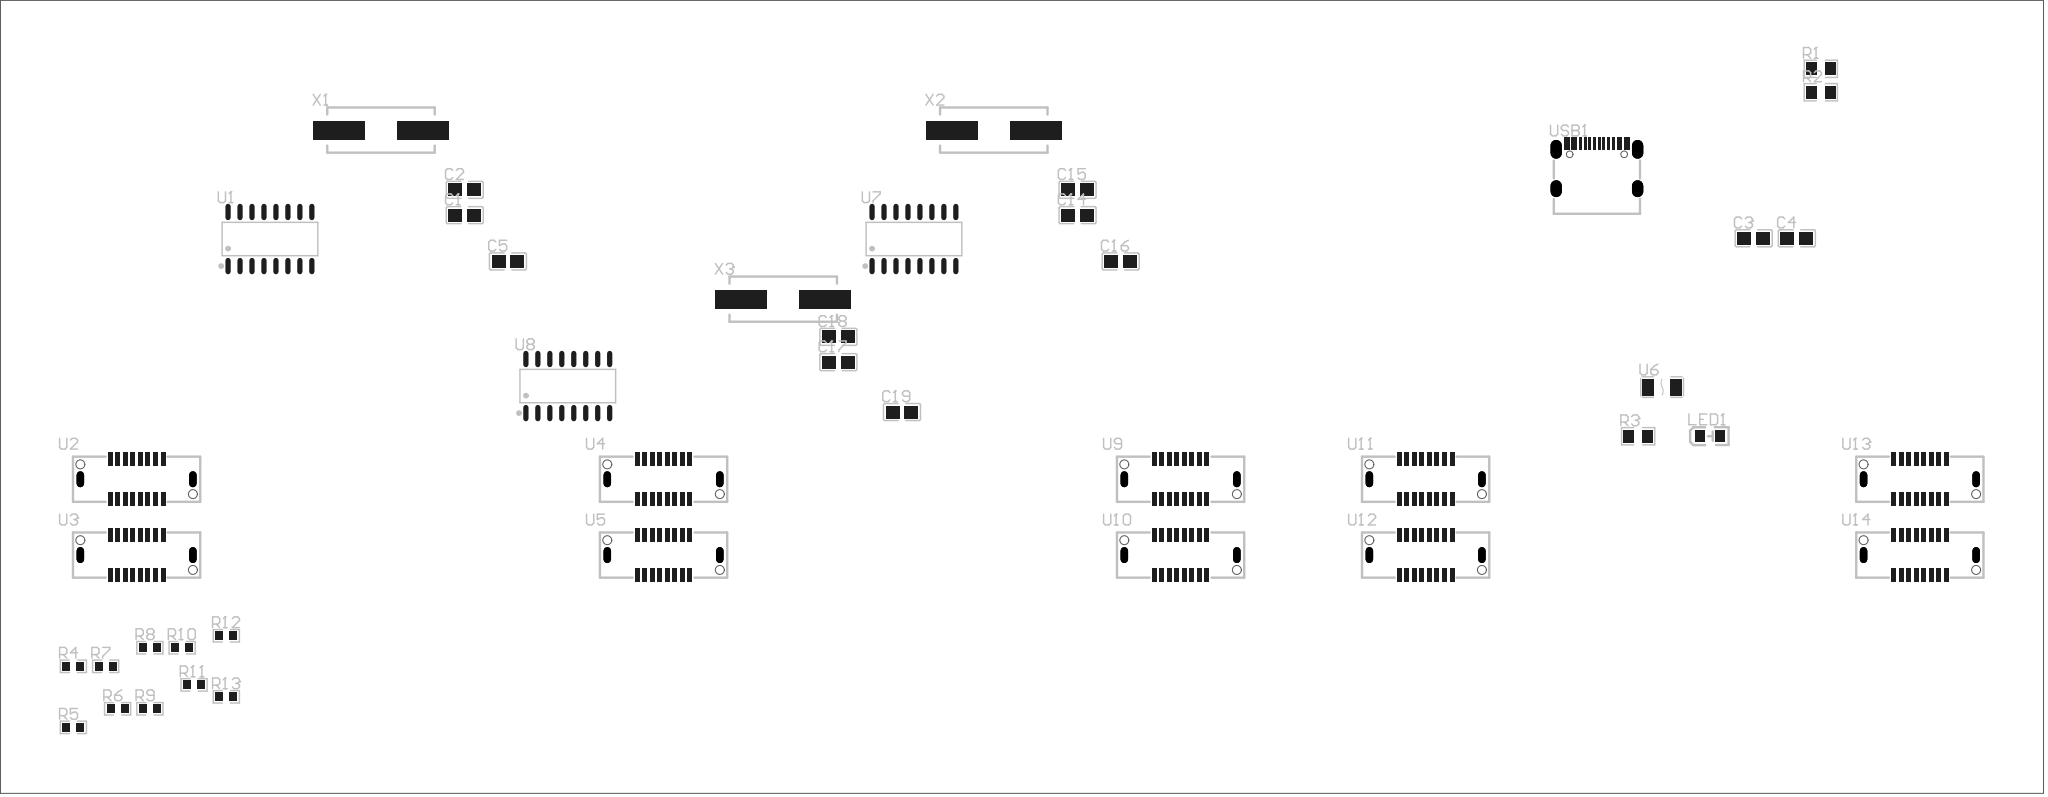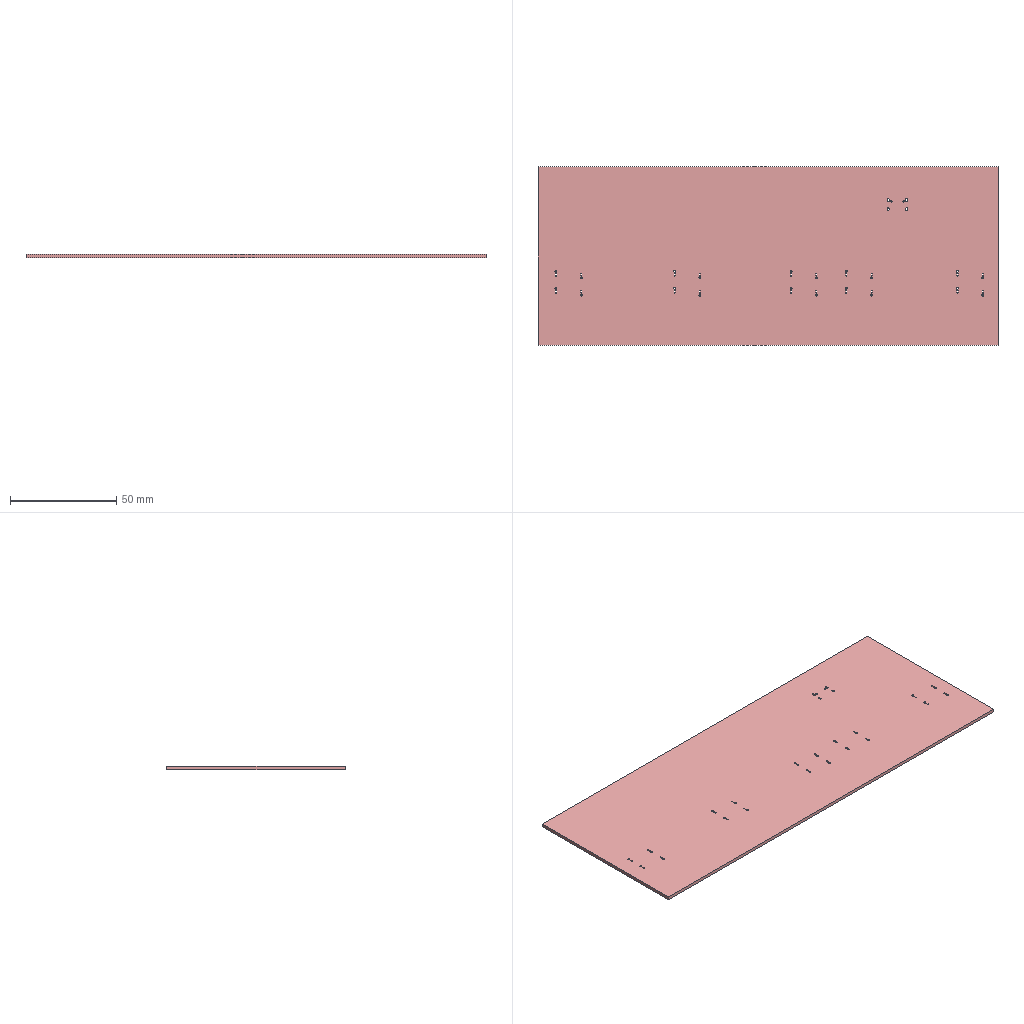Circuit board layout | Altium Designer | box 216.8 x 84.2 x 1.6 mm
Layer stack:
# Altium Designer layer stack of  (unit mm; dielectric type: 0 none, 1 core, 2 prepreg, 3 surface material)
index,name,kind,layer,copper_thickness_mm,dielectric_type,dielectric_thickness_mm,dielectric_material,dielectric_constant
0,Top Paste Mask Layer,other,,,,,,
1,Top Silkscreen Layer,other,,,,,,
2,Top Solder Mask Layer,dielectric,,,3,0.01,,3.3
3,Top Layer,copper,Top Layer,0.035,,,,
4,Dielectric1,dielectric,,,3,1.51,FR4,4.5
5,Bottom Layer,copper,Bottom Layer,0.035,,,,
6,Bottom Solder Mask Layer,dielectric,,,3,0.01,,3.3
7,Bottom Silkscreen Layer,other,,,,,,
8,Bottom Paste Mask Layer,other,,,,,,
# drill layer pairs: low layer,high layer
drill_pair,Top Layer,Bottom Layer
Part placement:
Designator,Comment,Layer,Footprint,Center-X(mm),Center-Y(mm),Rotation
C1,100nF,TopLayer,C0805,119.111,131.274,0
C2,100nF,TopLayer,C0805,119.111,133.959,0
C3,10UF,TopLayer,C0805,255.864,128.815,0
C4,0.1UF,TopLayer,C0805,260.443,128.815,0
C5,0.1UF,TopLayer,C0805,123.69,126.355,0
C14,100nF,TopLayer,C0805,184.127,131.274,0
C15,100nF,TopLayer,C0805,184.127,133.959,0
C16,0.1UF,TopLayer,C0805,188.706,126.355,0
C17,100nF,TopLayer,C0805,158.75,115.657,0
C18,100nF,TopLayer,C0805,158.75,118.341,0
C19,0.1UF,TopLayer,C0805,165.497,110.359,0
LED1,,TopLayer,LED_0805,251.217,107.793,0
R1,5.1K,TopLayer,R0805,262.983,146.816,0
R2,5.1K,TopLayer,R0805,262.983,144.329,0
R3,2K,TopLayer,R0805,243.605,107.788,0
U1,SL2.1A,TopLayer,SOP-16_L10.0-W3.9-P1.27-LS6.0-BL,98.441,128.734,0
U6,1.5A快恢复保险丝-1206,TopLayer,F1206,246.145,113.008,0
U7,SL2.1A,TopLayer,SOP-16_L10.0-W3.9-P1.27-LS6.0-BL,166.767,128.734,0
U8,SL2.1A,TopLayer,SOP-16_L10.0-W3.9-P1.27-LS6.0-BL,130.04,113.117,0
USB1,typec,TopLayer,USB-C-SMD_KH-TYPE-C-16P,239.228,136.499,0
X1,12MHz,TopLayer,CRYSTAL-SMD_L11.1-W4.8-LS12.3,110.221,140.309,0
X2,12MHz,TopLayer,CRYSTAL-SMD_L11.1-W4.8-LS12.3,175.237,140.309,0
X3,12MHz,TopLayer,CRYSTAL-SMD_L11.1-W4.8-LS12.3,152.9,122.348,0
U2,EZ-USBC-1143C,TopLayer,USB-SMD_EZ-USBC-1143C,84.294,103.217,0
U3,EZ-USBC-1143C,TopLayer,USB-SMD_EZ-USBC-1143C,84.294,95.163,0
U4,EZ-USBC-1143C,TopLayer,USB-SMD_EZ-USBC-1143C,140.2,103.217,0
U5,EZ-USBC-1143C,TopLayer,USB-SMD_EZ-USBC-1143C,140.2,95.163,0
U9,EZ-USBC-1143C,TopLayer,USB-SMD_EZ-USBC-1143C,195.056,103.217,0
U10,EZ-USBC-1143C,TopLayer,USB-SMD_EZ-USBC-1143C,195.056,95.163,0
U11,EZ-USBC-1143C,TopLayer,USB-SMD_EZ-USBC-1143C,221.055,103.217,0
U12,EZ-USBC-1143C,TopLayer,USB-SMD_EZ-USBC-1143C,221.055,95.163,0
U13,EZ-USBC-1143C,TopLayer,USB-SMD_EZ-USBC-1143C,273.49,103.217,0
U14,EZ-USBC-1143C,TopLayer,USB-SMD_EZ-USBC-1143C,273.49,95.163,0
R4,10K,TopLayer,R0603,77.585,83.348,0
R5,10K,TopLayer,R0603,77.585,76.861,0
R6,10K,TopLayer,R0603,82.278,78.834,0
R7,10K,TopLayer,R0603,81.008,83.348,0
R8,10K,TopLayer,R0603,85.7,85.321,0
R9,10K,TopLayer,R0603,85.7,78.834,0
R10,10K,TopLayer,R0603,89.123,85.321,0
R11,10K,TopLayer,R0603,90.393,81.374,0
R12,10K,TopLayer,R0603,93.815,86.591,0
R13,10K,TopLayer,R0603,93.815,80.104,0
Pad and via stacks:
# Altium Designer via and pad stacks of  (unit mm). Each distinct definition once, with the count of objects using it.
# via: kind,start_layer,end_layer,hole_mm,diameter_mm,mode(0 simple;1 top-mid-bottom;2 full stack),diameter_per_layer,count,example_net
# pad: kind,layer,hole_mm,hole_type(0 round;1 square;2 slot),plating,top_size,top_shape(1 round;2 rect;3 octagon;9 rounded rect),mid_size,bottom_size,mode,footprint,size_per_layer,count,example
pad,Top Layer,0,0,plated,1.41x1.35,2,1.41x1.35,1.41x1.35,0,C0805,,22,C1.2
pad,Top Layer,0,0,plated,1x1.25,2,1x1.25,1x1.25,0,LED_0805,,2,LED1.2
pad,Top Layer,0,0,plated,1.133x1.377,2,1.133x1.377,1.133x1.377,0,R0805,,6,R1.2
pad,Top Layer,0,0,plated,0.56x1.745,1,0.56x1.745,0.56x1.745,0,SOP-16_L10.0-W3.9-P1.27-LS6.0-BL,,48,U1.1
pad,Top Layer,0,0,plated,1.19x1.728,2,1.19x1.728,1.19x1.728,0,F1206,,2,U6.1
pad,Top Layer,0,0,plated,0.3x1.3,2,0.3x1.3,0.3x1.3,0,USB-C-SMD_KH-TYPE-C-16P,,16,USB1.A1
pad,Top Layer,0,0,plated,5.5x2,2,5.5x2,5.5x2,0,CRYSTAL-SMD_L11.1-W4.8-LS12.3,,6,X1.2
pad,Top Layer,0,0,plated,0.5x1.4,2,0.5x1.4,0.5x1.4,0,USB-SMD_EZ-USBC-1143C,,160,U2.A1
pad,Top Layer,0,0,plated,0.8065x0.864,2,0.8065x0.864,0.8065x0.864,0,R0603,,20,R4.2
pad,Multi-Layer,0.7,2,plated,1.2x1.8,1,1.2x1.8,1.2x1.8,0,USB-C-SMD_KH-TYPE-C-16P,,2,USB1.3
pad,Multi-Layer,0.7,2,plated,1.2x2,1,1.2x2,1.2x2,0,USB-C-SMD_KH-TYPE-C-16P,,2,USB1.2
pad,Multi-Layer,0.5,2,plated,0.8x1.7,1,0.8x1.7,0.8x1.7,0,USB-SMD_EZ-USBC-1143C,,20,U2.18
Design rules, without the lines most boards share:
# Altium Designer design rules of  (exported by Altium Designer, unit mm)
# columns: name | kind | enabled | priority | scope1 | scope2 | descriptor | typed fields (field=value)
copperThickness2oz | 0 | disabled | 1 | All | All | Clearance Constraint (Gap=6mil) (Disabled)(All),(All) | gap=0.1524
Plane_innerPlane | 0 | disabled | 2 | All | All | Clearance Constraint (Gap=6mil) (Disabled)(All),(All) | gap=0.1524
Copper_copperRegion | 0 | disabled | 3 | All | All | Clearance Constraint (Gap=6mil) (Disabled)(All),(All) | gap=0.1524
copperThickness1oz | 0 | enabled | 4 | All | All | Clearance Constraint (Gap=6mil) (All),(All) | gap=0.1524
otherClearance | 52 | enabled | 1 | All | All | Hole To Hole Clearance (Gap=11.8mil) (All),(All) | gap=0.2997
viaSize | 11 | enabled | 1 | All | All | Routing Via (MinHoleWidth=11.8mil) (MaxHoleWidth=248mil) (PreferredHoleWidth=12mil) (MinWidth=19.7mil) (MaxWidth=393.7mil) (PreferedWidth=24mil) (All) | via_min_hole=0.2997 via_max_hole=6.299 via_preferred_diameter=0.6096 via_preferred_hole=0.3048